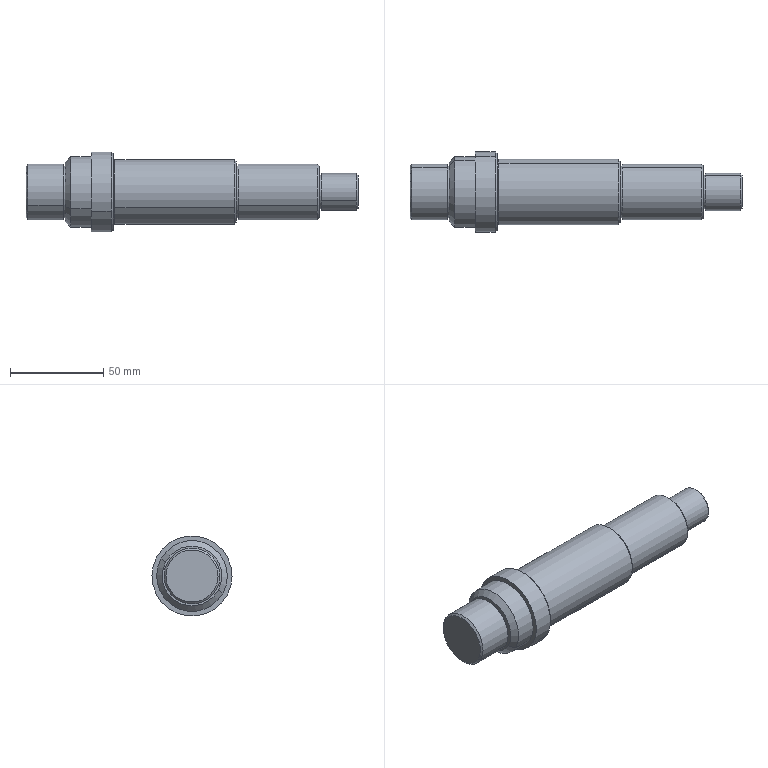Part | STEP file | 20316-1 | 1 solid | 43 faces | box 178 x 43 x 43 mm | volume 148101 mm3 | cylinder 20 | cone 12 | plane 11 | commonest cylinder face diameters 28 x4 30 x4 18 x2 20 x2 33 x2 35 x2
STEP:
#1=CARTESIAN_POINT('',(-19.8,7.898,4.315));
#2=VERTEX_POINT('',#1);
#3=CARTESIAN_POINT('',(-19.8,-7.898,-4.315));
#4=VERTEX_POINT('',#3);
#5=CARTESIAN_POINT('',(-19.8,0.,0.));
#6=DIRECTION('',(1.,0.,0.));
#7=AXIS2_PLACEMENT_3D('',#5,#6,$);
#8=CIRCLE('',#7,9.);
#9=EDGE_CURVE('',#2,#4,#8,.T.);
#10=ORIENTED_EDGE('',*,*,#9,.F.);
#11=CARTESIAN_POINT('',(-20.8,7.898,4.315));
#12=VERTEX_POINT('',#11);
#13=CARTESIAN_POINT('',(-20.3,7.898,4.315));
#14=DIRECTION('',(1.,0.,0.));
#15=VECTOR('',#14,1.);
#16=LINE('',#13,#15);
#17=EDGE_CURVE('',#2,#12,#16,.F.);
#18=ORIENTED_EDGE('',*,*,#17,.T.);
#19=CARTESIAN_POINT('',(-20.8,-7.898,-4.315));
#20=VERTEX_POINT('',#19);
#21=CARTESIAN_POINT('',(-20.8,0.,0.));
#22=DIRECTION('',(1.,0.,0.));
#23=AXIS2_PLACEMENT_3D('',#21,#22,$);
#24=CIRCLE('',#23,9.);
#25=EDGE_CURVE('',#12,#20,#24,.T.);
#26=ORIENTED_EDGE('',*,*,#25,.T.);
#27=CARTESIAN_POINT('',(-20.3,-7.898,-4.315));
#28=DIRECTION('',(1.,0.,0.));
#29=VECTOR('',#28,1.);
#30=LINE('',#27,#29);
#31=EDGE_CURVE('',#4,#20,#30,.F.);
#32=ORIENTED_EDGE('',*,*,#31,.F.);
#33=EDGE_LOOP('',(#10,#18,#26,#32));
#34=FACE_OUTER_BOUND('',#33,.T.);
#35=CARTESIAN_POINT('',(-89.,0.,0.));
#36=DIRECTION('',(1.,0.,0.));
#37=DIRECTION('',(0.,0.8776,0.4794));
#38=AXIS2_PLACEMENT_3D('',#35,#36,#37);
#39=CYLINDRICAL_SURFACE('',#38,9.);
#40=ADVANCED_FACE('',(#34),#39,.T.);
#41=CARTESIAN_POINT('',(-19.8,0.,0.));
#42=DIRECTION('',(1.,0.,0.));
#43=AXIS2_PLACEMENT_3D('',#41,#42,$);
#44=CIRCLE('',#43,9.);
#45=EDGE_CURVE('',#4,#2,#44,.T.);
#46=ORIENTED_EDGE('',*,*,#45,.F.);
#47=ORIENTED_EDGE('',*,*,#31,.T.);
#48=CARTESIAN_POINT('',(-20.8,0.,0.));
#49=DIRECTION('',(1.,0.,0.));
#50=AXIS2_PLACEMENT_3D('',#48,#49,$);
#51=CIRCLE('',#50,9.);
#52=EDGE_CURVE('',#20,#12,#51,.T.);
#53=ORIENTED_EDGE('',*,*,#52,.T.);
#54=ORIENTED_EDGE('',*,*,#17,.F.);
#55=EDGE_LOOP('',(#46,#47,#53,#54));
#56=FACE_OUTER_BOUND('',#55,.T.);
#57=ADVANCED_FACE('',(#56),#39,.T.);
#58=CARTESIAN_POINT('',(-64.3,12.286,6.712));
#59=VERTEX_POINT('',#58);
#60=CARTESIAN_POINT('',(-64.3,-12.286,-6.712));
#61=VERTEX_POINT('',#60);
#62=CARTESIAN_POINT('',(-64.3,0.,0.));
#63=DIRECTION('',(1.,0.,0.));
#64=AXIS2_PLACEMENT_3D('',#62,#63,$);
#65=CIRCLE('',#64,14.);
#66=EDGE_CURVE('',#59,#61,#65,.T.);
#67=ORIENTED_EDGE('',*,*,#66,.F.);
#68=CARTESIAN_POINT('',(-65.3,12.286,6.712));
#69=VERTEX_POINT('',#68);
#70=CARTESIAN_POINT('',(-111.15,12.286,6.712));
#71=DIRECTION('',(1.,0.,0.));
#72=VECTOR('',#71,1.);
#73=LINE('',#70,#72);
#74=EDGE_CURVE('',#59,#69,#73,.F.);
#75=ORIENTED_EDGE('',*,*,#74,.T.);
#76=CARTESIAN_POINT('',(-65.3,-12.286,-6.712));
#77=VERTEX_POINT('',#76);
#78=CARTESIAN_POINT('',(-65.3,0.,0.));
#79=DIRECTION('',(1.,0.,0.));
#80=AXIS2_PLACEMENT_3D('',#78,#79,$);
#81=CIRCLE('',#80,14.);
#82=EDGE_CURVE('',#69,#77,#81,.T.);
#83=ORIENTED_EDGE('',*,*,#82,.T.);
#84=CARTESIAN_POINT('',(-111.15,-12.286,-6.712));
#85=DIRECTION('',(1.,0.,0.));
#86=VECTOR('',#85,1.);
#87=LINE('',#84,#86);
#88=EDGE_CURVE('',#61,#77,#87,.F.);
#89=ORIENTED_EDGE('',*,*,#88,.F.);
#90=EDGE_LOOP('',(#67,#75,#83,#89));
#91=FACE_OUTER_BOUND('',#90,.T.);
#92=CARTESIAN_POINT('',(-89.,0.,0.));
#93=DIRECTION('',(1.,0.,0.));
#94=DIRECTION('',(0.,0.8776,0.4794));
#95=AXIS2_PLACEMENT_3D('',#92,#93,#94);
#96=CYLINDRICAL_SURFACE('',#95,14.);
#97=ADVANCED_FACE('',(#91),#96,.T.);
#98=CARTESIAN_POINT('',(-64.3,0.,0.));
#99=DIRECTION('',(1.,0.,0.));
#100=AXIS2_PLACEMENT_3D('',#98,#99,$);
#101=CIRCLE('',#100,14.);
#102=EDGE_CURVE('',#61,#59,#101,.T.);
#103=ORIENTED_EDGE('',*,*,#102,.F.);
#104=ORIENTED_EDGE('',*,*,#88,.T.);
#105=CARTESIAN_POINT('',(-65.3,0.,0.));
#106=DIRECTION('',(1.,0.,0.));
#107=AXIS2_PLACEMENT_3D('',#105,#106,$);
#108=CIRCLE('',#107,14.);
#109=EDGE_CURVE('',#77,#69,#108,.T.);
#110=ORIENTED_EDGE('',*,*,#109,.T.);
#111=ORIENTED_EDGE('',*,*,#74,.F.);
#112=EDGE_LOOP('',(#103,#104,#110,#111));
#113=FACE_OUTER_BOUND('',#112,.T.);
#114=ADVANCED_FACE('',(#113),#96,.T.);
#115=CARTESIAN_POINT('',(-130.3,14.48,7.911));
#116=VERTEX_POINT('',#115);
#117=CARTESIAN_POINT('',(-130.3,-14.48,-7.911));
#118=VERTEX_POINT('',#117);
#119=CARTESIAN_POINT('',(-130.3,0.,0.));
#120=DIRECTION('',(1.,0.,0.));
#121=AXIS2_PLACEMENT_3D('',#119,#120,$);
#122=CIRCLE('',#121,16.5);
#123=EDGE_CURVE('',#116,#118,#122,.T.);
#124=ORIENTED_EDGE('',*,*,#123,.F.);
#125=CARTESIAN_POINT('',(-131.3,14.48,7.911));
#126=VERTEX_POINT('',#125);
#127=CARTESIAN_POINT('',(-130.8,14.48,7.911));
#128=DIRECTION('',(1.,0.,0.));
#129=VECTOR('',#128,1.);
#130=LINE('',#127,#129);
#131=EDGE_CURVE('',#116,#126,#130,.F.);
#132=ORIENTED_EDGE('',*,*,#131,.T.);
#133=CARTESIAN_POINT('',(-131.3,-14.48,-7.911));
#134=VERTEX_POINT('',#133);
#135=CARTESIAN_POINT('',(-131.3,0.,0.));
#136=DIRECTION('',(1.,0.,0.));
#137=AXIS2_PLACEMENT_3D('',#135,#136,$);
#138=CIRCLE('',#137,16.5);
#139=EDGE_CURVE('',#126,#134,#138,.T.);
#140=ORIENTED_EDGE('',*,*,#139,.T.);
#141=CARTESIAN_POINT('',(-130.8,-14.48,-7.911));
#142=DIRECTION('',(1.,0.,0.));
#143=VECTOR('',#142,1.);
#144=LINE('',#141,#143);
#145=EDGE_CURVE('',#118,#134,#144,.F.);
#146=ORIENTED_EDGE('',*,*,#145,.F.);
#147=EDGE_LOOP('',(#124,#132,#140,#146));
#148=FACE_OUTER_BOUND('',#147,.T.);
#149=CARTESIAN_POINT('',(-89.,0.,0.));
#150=DIRECTION('',(1.,0.,0.));
#151=DIRECTION('',(0.,0.8776,0.4794));
#152=AXIS2_PLACEMENT_3D('',#149,#150,#151);
#153=CYLINDRICAL_SURFACE('',#152,16.5);
#154=ADVANCED_FACE('',(#148),#153,.T.);
#155=CARTESIAN_POINT('',(-130.3,0.,0.));
#156=DIRECTION('',(1.,0.,0.));
#157=AXIS2_PLACEMENT_3D('',#155,#156,$);
#158=CIRCLE('',#157,16.5);
#159=EDGE_CURVE('',#118,#116,#158,.T.);
#160=ORIENTED_EDGE('',*,*,#159,.F.);
#161=ORIENTED_EDGE('',*,*,#145,.T.);
#162=CARTESIAN_POINT('',(-131.3,0.,0.));
#163=DIRECTION('',(1.,0.,0.));
#164=AXIS2_PLACEMENT_3D('',#162,#163,$);
#165=CIRCLE('',#164,16.5);
#166=EDGE_CURVE('',#134,#126,#165,.T.);
#167=ORIENTED_EDGE('',*,*,#166,.T.);
#168=ORIENTED_EDGE('',*,*,#131,.F.);
#169=EDGE_LOOP('',(#160,#161,#167,#168));
#170=FACE_OUTER_BOUND('',#169,.T.);
#171=ADVANCED_FACE('',(#170),#153,.T.);
#172=CARTESIAN_POINT('',(-157.,12.286,6.712));
#173=VERTEX_POINT('',#172);
#174=CARTESIAN_POINT('',(-157.,-12.286,-6.712));
#175=VERTEX_POINT('',#174);
#176=CARTESIAN_POINT('',(-157.,0.,0.));
#177=DIRECTION('',(1.,0.,0.));
#178=AXIS2_PLACEMENT_3D('',#176,#177,$);
#179=CIRCLE('',#178,14.);
#180=EDGE_CURVE('',#173,#175,#179,.T.);
#181=ORIENTED_EDGE('',*,*,#180,.F.);
#182=CARTESIAN_POINT('',(-158.,12.286,6.712));
#183=VERTEX_POINT('',#182);
#184=CARTESIAN_POINT('',(-111.15,12.286,6.712));
#185=DIRECTION('',(1.,0.,0.));
#186=VECTOR('',#185,1.);
#187=LINE('',#184,#186);
#188=EDGE_CURVE('',#173,#183,#187,.F.);
#189=ORIENTED_EDGE('',*,*,#188,.T.);
#190=CARTESIAN_POINT('',(-158.,-12.286,-6.712));
#191=VERTEX_POINT('',#190);
#192=CARTESIAN_POINT('',(-158.,0.,0.));
#193=DIRECTION('',(1.,0.,0.));
#194=AXIS2_PLACEMENT_3D('',#192,#193,$);
#195=CIRCLE('',#194,14.);
#196=EDGE_CURVE('',#183,#191,#195,.T.);
#197=ORIENTED_EDGE('',*,*,#196,.T.);
#198=CARTESIAN_POINT('',(-111.15,-12.286,-6.712));
#199=DIRECTION('',(1.,0.,0.));
#200=VECTOR('',#199,1.);
#201=LINE('',#198,#200);
#202=EDGE_CURVE('',#175,#191,#201,.F.);
#203=ORIENTED_EDGE('',*,*,#202,.F.);
#204=EDGE_LOOP('',(#181,#189,#197,#203));
#205=FACE_OUTER_BOUND('',#204,.T.);
#206=ADVANCED_FACE('',(#205),#96,.T.);
#207=CARTESIAN_POINT('',(-157.,0.,0.));
#208=DIRECTION('',(1.,0.,0.));
#209=AXIS2_PLACEMENT_3D('',#207,#208,$);
#210=CIRCLE('',#209,14.);
#211=EDGE_CURVE('',#175,#173,#210,.T.);
#212=ORIENTED_EDGE('',*,*,#211,.F.);
#213=ORIENTED_EDGE('',*,*,#202,.T.);
#214=CARTESIAN_POINT('',(-158.,0.,0.));
#215=DIRECTION('',(1.,0.,0.));
#216=AXIS2_PLACEMENT_3D('',#214,#215,$);
#217=CIRCLE('',#216,14.);
#218=EDGE_CURVE('',#191,#183,#217,.T.);
#219=ORIENTED_EDGE('',*,*,#218,.T.);
#220=ORIENTED_EDGE('',*,*,#188,.F.);
#221=EDGE_LOOP('',(#212,#213,#219,#220));
#222=FACE_OUTER_BOUND('',#221,.T.);
#223=ADVANCED_FACE('',(#222),#96,.T.);
#224=CARTESIAN_POINT('',(-19.8,8.776,4.794));
#225=VERTEX_POINT('',#224);
#226=CARTESIAN_POINT('',(-19.8,-8.776,-4.794));
#227=VERTEX_POINT('',#226);
#228=CARTESIAN_POINT('',(-19.8,0.,0.));
#229=DIRECTION('',(1.,0.,0.));
#230=AXIS2_PLACEMENT_3D('',#228,#229,$);
#231=CIRCLE('',#230,10.);
#232=EDGE_CURVE('',#225,#227,#231,.T.);
#233=ORIENTED_EDGE('',*,*,#232,.F.);
#234=CARTESIAN_POINT('',(-19.8,0.,0.));
#235=DIRECTION('',(1.,0.,0.));
#236=AXIS2_PLACEMENT_3D('',#234,#235,$);
#237=CIRCLE('',#236,10.);
#238=EDGE_CURVE('',#227,#225,#237,.T.);
#239=ORIENTED_EDGE('',*,*,#238,.F.);
#240=EDGE_LOOP('',(#233,#239));
#241=FACE_OUTER_BOUND('',#240,.T.);
#242=ORIENTED_EDGE('',*,*,#45,.T.);
#243=ORIENTED_EDGE('',*,*,#9,.T.);
#244=EDGE_LOOP('',(#242,#243));
#245=FACE_BOUND('',#244,.T.);
#246=CARTESIAN_POINT('',(-19.8,10.,0.));
#247=DIRECTION('',(1.,0.,0.));
#248=DIRECTION('',(0.,1.,0.));
#249=AXIS2_PLACEMENT_3D('',#246,#247,#248);
#250=PLANE('',#249);
#251=ADVANCED_FACE('',(#241,#245),#250,.F.);
#252=CARTESIAN_POINT('',(-64.3,13.164,7.191));
#253=VERTEX_POINT('',#252);
#254=CARTESIAN_POINT('',(-64.3,-13.164,-7.191));
#255=VERTEX_POINT('',#254);
#256=CARTESIAN_POINT('',(-64.3,0.,0.));
#257=DIRECTION('',(1.,0.,0.));
#258=AXIS2_PLACEMENT_3D('',#256,#257,$);
#259=CIRCLE('',#258,15.);
#260=EDGE_CURVE('',#253,#255,#259,.T.);
#261=ORIENTED_EDGE('',*,*,#260,.F.);
#262=CARTESIAN_POINT('',(-64.3,0.,0.));
#263=DIRECTION('',(1.,0.,0.));
#264=AXIS2_PLACEMENT_3D('',#262,#263,$);
#265=CIRCLE('',#264,15.);
#266=EDGE_CURVE('',#255,#253,#265,.T.);
#267=ORIENTED_EDGE('',*,*,#266,.F.);
#268=EDGE_LOOP('',(#261,#267));
#269=FACE_OUTER_BOUND('',#268,.T.);
#270=ORIENTED_EDGE('',*,*,#102,.T.);
#271=ORIENTED_EDGE('',*,*,#66,.T.);
#272=EDGE_LOOP('',(#270,#271));
#273=FACE_BOUND('',#272,.T.);
#274=CARTESIAN_POINT('',(-64.3,15.,0.));
#275=DIRECTION('',(1.,0.,0.));
#276=DIRECTION('',(0.,1.,0.));
#277=AXIS2_PLACEMENT_3D('',#274,#275,#276);
#278=PLANE('',#277);
#279=ADVANCED_FACE('',(#269,#273),#278,.F.);
#280=CARTESIAN_POINT('',(-130.3,15.358,8.39));
#281=VERTEX_POINT('',#280);
#282=CARTESIAN_POINT('',(-130.3,-15.358,-8.39));
#283=VERTEX_POINT('',#282);
#284=CARTESIAN_POINT('',(-130.3,0.,0.));
#285=DIRECTION('',(1.,0.,0.));
#286=AXIS2_PLACEMENT_3D('',#284,#285,$);
#287=CIRCLE('',#286,17.5);
#288=EDGE_CURVE('',#281,#283,#287,.T.);
#289=ORIENTED_EDGE('',*,*,#288,.F.);
#290=CARTESIAN_POINT('',(-130.3,0.,0.));
#291=DIRECTION('',(1.,0.,0.));
#292=AXIS2_PLACEMENT_3D('',#290,#291,$);
#293=CIRCLE('',#292,17.5);
#294=EDGE_CURVE('',#283,#281,#293,.T.);
#295=ORIENTED_EDGE('',*,*,#294,.F.);
#296=EDGE_LOOP('',(#289,#295));
#297=FACE_OUTER_BOUND('',#296,.T.);
#298=ORIENTED_EDGE('',*,*,#159,.T.);
#299=ORIENTED_EDGE('',*,*,#123,.T.);
#300=EDGE_LOOP('',(#298,#299));
#301=FACE_BOUND('',#300,.T.);
#302=CARTESIAN_POINT('',(-130.3,17.5,0.));
#303=DIRECTION('',(1.,0.,0.));
#304=DIRECTION('',(0.,1.,0.));
#305=AXIS2_PLACEMENT_3D('',#302,#303,#304);
#306=PLANE('',#305);
#307=ADVANCED_FACE('',(#297,#301),#306,.F.);
#308=CARTESIAN_POINT('',(-143.,18.868,10.308));
#309=VERTEX_POINT('',#308);
#310=CARTESIAN_POINT('',(-143.,-18.868,-10.308));
#311=VERTEX_POINT('',#310);
#312=CARTESIAN_POINT('',(-143.,0.,0.));
#313=DIRECTION('',(1.,0.,0.));
#314=AXIS2_PLACEMENT_3D('',#312,#313,$);
#315=CIRCLE('',#314,21.5);
#316=EDGE_CURVE('',#309,#311,#315,.T.);
#317=ORIENTED_EDGE('',*,*,#316,.F.);
#318=CARTESIAN_POINT('',(-143.,0.,0.));
#319=DIRECTION('',(1.,0.,0.));
#320=AXIS2_PLACEMENT_3D('',#318,#319,$);
#321=CIRCLE('',#320,21.5);
#322=EDGE_CURVE('',#311,#309,#321,.T.);
#323=ORIENTED_EDGE('',*,*,#322,.F.);
#324=EDGE_LOOP('',(#317,#323));
#325=FACE_OUTER_BOUND('',#324,.T.);
#326=CARTESIAN_POINT('',(-143.,-16.674,-9.109));
#327=VERTEX_POINT('',#326);
#328=CARTESIAN_POINT('',(-143.,16.674,9.109));
#329=VERTEX_POINT('',#328);
#330=CARTESIAN_POINT('',(-143.,0.,0.));
#331=DIRECTION('',(1.,0.,0.));
#332=AXIS2_PLACEMENT_3D('',#330,#331,$);
#333=CIRCLE('',#332,19.);
#334=EDGE_CURVE('',#327,#329,#333,.T.);
#335=ORIENTED_EDGE('',*,*,#334,.T.);
#336=CARTESIAN_POINT('',(-143.,0.,0.));
#337=DIRECTION('',(1.,0.,0.));
#338=AXIS2_PLACEMENT_3D('',#336,#337,$);
#339=CIRCLE('',#338,19.);
#340=EDGE_CURVE('',#329,#327,#339,.T.);
#341=ORIENTED_EDGE('',*,*,#340,.T.);
#342=EDGE_LOOP('',(#335,#341));
#343=FACE_BOUND('',#342,.T.);
#344=CARTESIAN_POINT('',(-143.,21.5,0.));
#345=DIRECTION('',(1.,0.,0.));
#346=DIRECTION('',(0.,1.,0.));
#347=AXIS2_PLACEMENT_3D('',#344,#345,#346);
#348=PLANE('',#347);
#349=ADVANCED_FACE('',(#325,#343),#348,.F.);
#350=CARTESIAN_POINT('',(-158.,-13.164,-7.191));
#351=VERTEX_POINT('',#350);
#352=CARTESIAN_POINT('',(-158.,13.164,7.191));
#353=VERTEX_POINT('',#352);
#354=CARTESIAN_POINT('',(-158.,0.,0.));
#355=DIRECTION('',(1.,0.,0.));
#356=AXIS2_PLACEMENT_3D('',#354,#355,$);
#357=CIRCLE('',#356,15.);
#358=EDGE_CURVE('',#351,#353,#357,.T.);
#359=ORIENTED_EDGE('',*,*,#358,.T.);
#360=CARTESIAN_POINT('',(-158.,0.,0.));
#361=DIRECTION('',(1.,0.,0.));
#362=AXIS2_PLACEMENT_3D('',#360,#361,$);
#363=CIRCLE('',#362,15.);
#364=EDGE_CURVE('',#353,#351,#363,.T.);
#365=ORIENTED_EDGE('',*,*,#364,.T.);
#366=EDGE_LOOP('',(#359,#365));
#367=FACE_OUTER_BOUND('',#366,.T.);
#368=ORIENTED_EDGE('',*,*,#196,.F.);
#369=ORIENTED_EDGE('',*,*,#218,.F.);
#370=EDGE_LOOP('',(#368,#369));
#371=FACE_BOUND('',#370,.T.);
#372=CARTESIAN_POINT('',(-158.,15.,0.));
#373=DIRECTION('',(1.,0.,0.));
#374=DIRECTION('',(0.,1.,0.));
#375=AXIS2_PLACEMENT_3D('',#372,#373,#374);
#376=PLANE('',#375);
#377=ADVANCED_FACE('',(#367,#371),#376,.T.);
#378=CARTESIAN_POINT('',(-177.,-13.164,-7.191));
#379=VERTEX_POINT('',#378);
#380=CARTESIAN_POINT('',(-99.4,-13.164,-7.191));
#381=DIRECTION('',(1.,0.,0.));
#382=VECTOR('',#381,1.);
#383=LINE('',#380,#382);
#384=EDGE_CURVE('',#351,#379,#383,.F.);
#385=ORIENTED_EDGE('',*,*,#384,.F.);
#386=ORIENTED_EDGE('',*,*,#364,.F.);
#387=CARTESIAN_POINT('',(-177.,13.164,7.191));
#388=VERTEX_POINT('',#387);
#389=CARTESIAN_POINT('',(-99.4,13.164,7.191));
#390=DIRECTION('',(1.,0.,0.));
#391=VECTOR('',#390,1.);
#392=LINE('',#389,#391);
#393=EDGE_CURVE('',#353,#388,#392,.F.);
#394=ORIENTED_EDGE('',*,*,#393,.T.);
#395=CARTESIAN_POINT('',(-177.,0.,0.));
#396=DIRECTION('',(1.,0.,0.));
#397=AXIS2_PLACEMENT_3D('',#395,#396,$);
#398=CIRCLE('',#397,15.);
#399=EDGE_CURVE('',#388,#379,#398,.T.);
#400=ORIENTED_EDGE('',*,*,#399,.T.);
#401=EDGE_LOOP('',(#385,#386,#394,#400));
#402=FACE_OUTER_BOUND('',#401,.T.);
#403=CARTESIAN_POINT('',(-89.,0.,0.));
#404=DIRECTION('',(1.,0.,0.));
#405=DIRECTION('',(0.,0.8776,0.4794));
#406=AXIS2_PLACEMENT_3D('',#403,#404,#405);
#407=CYLINDRICAL_SURFACE('',#406,15.);
#408=ADVANCED_FACE('',(#402),#407,.T.);
#409=ORIENTED_EDGE('',*,*,#393,.F.);
#410=ORIENTED_EDGE('',*,*,#358,.F.);
#411=ORIENTED_EDGE('',*,*,#384,.T.);
#412=CARTESIAN_POINT('',(-177.,0.,0.));
#413=DIRECTION('',(1.,0.,0.));
#414=AXIS2_PLACEMENT_3D('',#412,#413,$);
#415=CIRCLE('',#414,15.);
#416=EDGE_CURVE('',#379,#388,#415,.T.);
#417=ORIENTED_EDGE('',*,*,#416,.T.);
#418=EDGE_LOOP('',(#409,#410,#411,#417));
#419=FACE_OUTER_BOUND('',#418,.T.);
#420=ADVANCED_FACE('',(#419),#407,.T.);
#421=CARTESIAN_POINT('',(-178.,12.286,6.712));
#422=VERTEX_POINT('',#421);
#423=CARTESIAN_POINT('',(-178.,-12.286,-6.712));
#424=VERTEX_POINT('',#423);
#425=CARTESIAN_POINT('',(-178.,0.,0.));
#426=DIRECTION('',(1.,0.,0.));
#427=AXIS2_PLACEMENT_3D('',#425,#426,$);
#428=CIRCLE('',#427,14.);
#429=EDGE_CURVE('',#422,#424,#428,.T.);
#430=ORIENTED_EDGE('',*,*,#429,.F.);
#431=CARTESIAN_POINT('',(-178.,0.,0.));
#432=DIRECTION('',(1.,0.,0.));
#433=AXIS2_PLACEMENT_3D('',#431,#432,$);
#434=CIRCLE('',#433,14.);
#435=EDGE_CURVE('',#424,#422,#434,.T.);
#436=ORIENTED_EDGE('',*,*,#435,.F.);
#437=EDGE_LOOP('',(#430,#436));
#438=FACE_OUTER_BOUND('',#437,.T.);
#439=CARTESIAN_POINT('',(-178.,15.,0.));
#440=DIRECTION('',(1.,0.,0.));
#441=DIRECTION('',(0.,1.,0.));
#442=AXIS2_PLACEMENT_3D('',#439,#440,#441);
#443=PLANE('',#442);
#444=ADVANCED_FACE('',(#438),#443,.F.);
#445=CARTESIAN_POINT('',(-177.5,-12.725,-6.952));
#446=DIRECTION('',(0.7071,-0.6205,-0.339));
#447=VECTOR('',#446,1.);
#448=LINE('',#445,#447);
#449=EDGE_CURVE('',#379,#424,#448,.F.);
#450=ORIENTED_EDGE('',*,*,#449,.T.);
#451=ORIENTED_EDGE('',*,*,#435,.T.);
#452=CARTESIAN_POINT('',(-177.5,12.725,6.952));
#453=DIRECTION('',(0.7071,0.6205,0.339));
#454=VECTOR('',#453,1.);
#455=LINE('',#452,#454);
#456=EDGE_CURVE('',#388,#422,#455,.F.);
#457=ORIENTED_EDGE('',*,*,#456,.F.);
#458=ORIENTED_EDGE('',*,*,#416,.F.);
#459=EDGE_LOOP('',(#450,#451,#457,#458));
#460=FACE_OUTER_BOUND('',#459,.T.);
#461=CARTESIAN_POINT('',(-192.,0.,0.));
#462=DIRECTION('',(1.,0.,0.));
#463=DIRECTION('',(0.,-0.8958,-0.4444));
#464=AXIS2_PLACEMENT_3D('',#461,#462,#463);
#465=CONICAL_SURFACE('',#464,0.,0.7854);
#466=ADVANCED_FACE('',(#460),#465,.T.);
#467=ORIENTED_EDGE('',*,*,#456,.T.);
#468=ORIENTED_EDGE('',*,*,#429,.T.);
#469=ORIENTED_EDGE('',*,*,#449,.F.);
#470=ORIENTED_EDGE('',*,*,#399,.F.);
#471=EDGE_LOOP('',(#467,#468,#469,#470));
#472=FACE_OUTER_BOUND('',#471,.T.);
#473=CARTESIAN_POINT('',(-192.,0.,0.));
#474=DIRECTION('',(1.,0.,0.));
#475=DIRECTION('',(0.,0.8776,0.4794));
#476=AXIS2_PLACEMENT_3D('',#473,#474,#475);
#477=CONICAL_SURFACE('',#476,0.,0.7854);
#478=ADVANCED_FACE('',(#472),#477,.T.);
#479=CARTESIAN_POINT('',(-132.3,18.868,10.308));
#480=VERTEX_POINT('',#479);
#481=CARTESIAN_POINT('',(-137.15,18.868,10.308));
#482=DIRECTION('',(1.,0.,0.));
#483=VECTOR('',#482,1.);
#484=LINE('',#481,#483);
#485=EDGE_CURVE('',#480,#309,#484,.F.);
#486=ORIENTED_EDGE('',*,*,#485,.T.);
#487=ORIENTED_EDGE('',*,*,#316,.T.);
#488=CARTESIAN_POINT('',(-132.3,-18.868,-10.308));
#489=VERTEX_POINT('',#488);
#490=CARTESIAN_POINT('',(-137.15,-18.868,-10.308));
#491=DIRECTION('',(1.,0.,0.));
#492=VECTOR('',#491,1.);
#493=LINE('',#490,#492);
#494=EDGE_CURVE('',#489,#311,#493,.F.);
#495=ORIENTED_EDGE('',*,*,#494,.F.);
#496=CARTESIAN_POINT('',(-132.3,0.,0.));
#497=DIRECTION('',(1.,0.,0.));
#498=AXIS2_PLACEMENT_3D('',#496,#497,$);
#499=CIRCLE('',#498,21.5);
#500=EDGE_CURVE('',#480,#489,#499,.T.);
#501=ORIENTED_EDGE('',*,*,#500,.F.);
#502=EDGE_LOOP('',(#486,#487,#495,#501));
#503=FACE_OUTER_BOUND('',#502,.T.);
#504=CARTESIAN_POINT('',(-89.,0.,0.));
#505=DIRECTION('',(1.,0.,0.));
#506=DIRECTION('',(0.,0.8776,0.4794));
#507=AXIS2_PLACEMENT_3D('',#504,#505,#506);
#508=CYLINDRICAL_SURFACE('',#507,21.5);
#509=ADVANCED_FACE('',(#503),#508,.T.);
#510=ORIENTED_EDGE('',*,*,#494,.T.);
#511=ORIENTED_EDGE('',*,*,#322,.T.);
#512=ORIENTED_EDGE('',*,*,#485,.F.);
#513=CARTESIAN_POINT('',(-132.3,0.,0.));
#514=DIRECTION('',(1.,0.,0.));
#515=AXIS2_PLACEMENT_3D('',#513,#514,$);
#516=CIRCLE('',#515,21.5);
#517=EDGE_CURVE('',#489,#480,#516,.T.);
#518=ORIENTED_EDGE('',*,*,#517,.F.);
#519=EDGE_LOOP('',(#510,#511,#512,#518));
#520=FACE_OUTER_BOUND('',#519,.T.);
#521=ADVANCED_FACE('',(#520),#508,.T.);
#522=CARTESIAN_POINT('',(-131.3,-17.99,-9.828));
#523=VERTEX_POINT('',#522);
#524=CARTESIAN_POINT('',(-131.3,17.99,9.828));
#525=VERTEX_POINT('',#524);
#526=CARTESIAN_POINT('',(-131.3,0.,0.));
#527=DIRECTION('',(1.,0.,0.));
#528=AXIS2_PLACEMENT_3D('',#526,#527,$);
#529=CIRCLE('',#528,20.5);
#530=EDGE_CURVE('',#523,#525,#529,.T.);
#531=ORIENTED_EDGE('',*,*,#530,.T.);
#532=CARTESIAN_POINT('',(-131.3,0.,0.));
#533=DIRECTION('',(1.,0.,0.));
#534=AXIS2_PLACEMENT_3D('',#532,#533,$);
#535=CIRCLE('',#534,20.5);
#536=EDGE_CURVE('',#525,#523,#535,.T.);
#537=ORIENTED_EDGE('',*,*,#536,.T.);
#538=EDGE_LOOP('',(#531,#537));
#539=FACE_OUTER_BOUND('',#538,.T.);
#540=ORIENTED_EDGE('',*,*,#139,.F.);
#541=ORIENTED_EDGE('',*,*,#166,.F.);
#542=EDGE_LOOP('',(#540,#541));
#543=FACE_BOUND('',#542,.T.);
#544=CARTESIAN_POINT('',(-131.3,16.5,0.));
#545=DIRECTION('',(1.,0.,0.));
#546=DIRECTION('',(0.,1.,0.));
#547=AXIS2_PLACEMENT_3D('',#544,#545,#546);
#548=PLANE('',#547);
#549=ADVANCED_FACE('',(#539,#543),#548,.T.);
#550=CARTESIAN_POINT('',(-131.8,-18.429,-10.068));
#551=DIRECTION('',(-0.7071,-0.6205,-0.339));
#552=VECTOR('',#551,1.);
#553=LINE('',#550,#552);
#554=EDGE_CURVE('',#523,#489,#553,.T.);
#555=ORIENTED_EDGE('',*,*,#554,.T.);
#556=ORIENTED_EDGE('',*,*,#517,.T.);
#557=CARTESIAN_POINT('',(-131.8,18.429,10.068));
#558=DIRECTION('',(-0.7071,0.6205,0.339));
#559=VECTOR('',#558,1.);
#560=LINE('',#557,#559);
#561=EDGE_CURVE('',#525,#480,#560,.T.);
#562=ORIENTED_EDGE('',*,*,#561,.F.);
#563=ORIENTED_EDGE('',*,*,#530,.F.);
#564=EDGE_LOOP('',(#555,#556,#562,#563));
#565=FACE_OUTER_BOUND('',#564,.T.);
#566=CARTESIAN_POINT('',(-110.8,0.,0.));
#567=DIRECTION('',(-1.,0.,0.));
#568=DIRECTION('',(0.,-0.9997,-0.0256));
#569=AXIS2_PLACEMENT_3D('',#566,#567,#568);
#570=CONICAL_SURFACE('',#569,0.,0.7854);
#571=ADVANCED_FACE('',(#565),#570,.T.);
#572=ORIENTED_EDGE('',*,*,#561,.T.);
#573=ORIENTED_EDGE('',*,*,#500,.T.);
#574=ORIENTED_EDGE('',*,*,#554,.F.);
#575=ORIENTED_EDGE('',*,*,#536,.F.);
#576=EDGE_LOOP('',(#572,#573,#574,#575));
#577=FACE_OUTER_BOUND('',#576,.T.);
#578=CARTESIAN_POINT('',(-110.8,0.,0.));
#579=DIRECTION('',(-1.,0.,0.));
#580=DIRECTION('',(0.,0.8776,0.4794));
#581=AXIS2_PLACEMENT_3D('',#578,#579,#580);
#582=CONICAL_SURFACE('',#581,0.,0.7854);
#583=ADVANCED_FACE('',(#577),#582,.T.);
#584=CARTESIAN_POINT('',(-66.3,15.358,8.39));
#585=VERTEX_POINT('',#584);
#586=CARTESIAN_POINT('',(-97.8,15.358,8.39));
#587=DIRECTION('',(1.,0.,0.));
#588=VECTOR('',#587,1.);
#589=LINE('',#586,#588);
#590=EDGE_CURVE('',#585,#281,#589,.F.);
#591=ORIENTED_EDGE('',*,*,#590,.T.);
#592=ORIENTED_EDGE('',*,*,#288,.T.);
#593=CARTESIAN_POINT('',(-66.3,-15.358,-8.39));
#594=VERTEX_POINT('',#593);
#595=CARTESIAN_POINT('',(-97.8,-15.358,-8.39));
#596=DIRECTION('',(1.,0.,0.));
#597=VECTOR('',#596,1.);
#598=LINE('',#595,#597);
#599=EDGE_CURVE('',#594,#283,#598,.F.);
#600=ORIENTED_EDGE('',*,*,#599,.F.);
#601=CARTESIAN_POINT('',(-66.3,0.,0.));
#602=DIRECTION('',(1.,0.,0.));
#603=AXIS2_PLACEMENT_3D('',#601,#602,$);
#604=CIRCLE('',#603,17.5);
#605=EDGE_CURVE('',#585,#594,#604,.T.);
#606=ORIENTED_EDGE('',*,*,#605,.F.);
#607=EDGE_LOOP('',(#591,#592,#600,#606));
#608=FACE_OUTER_BOUND('',#607,.T.);
#609=CARTESIAN_POINT('',(-89.,0.,0.));
#610=DIRECTION('',(1.,0.,0.));
#611=DIRECTION('',(0.,0.8776,0.4794));
#612=AXIS2_PLACEMENT_3D('',#609,#610,#611);
#613=CYLINDRICAL_SURFACE('',#612,17.5);
#614=ADVANCED_FACE('',(#608),#613,.T.);
#615=ORIENTED_EDGE('',*,*,#599,.T.);
#616=ORIENTED_EDGE('',*,*,#294,.T.);
#617=ORIENTED_EDGE('',*,*,#590,.F.);
#618=CARTESIAN_POINT('',(-66.3,0.,0.));
#619=DIRECTION('',(1.,0.,0.));
#620=AXIS2_PLACEMENT_3D('',#618,#619,$);
#621=CIRCLE('',#620,17.5);
#622=EDGE_CURVE('',#594,#585,#621,.T.);
#623=ORIENTED_EDGE('',*,*,#622,.F.);
#624=EDGE_LOOP('',(#615,#616,#617,#623));
#625=FACE_OUTER_BOUND('',#624,.T.);
#626=ADVANCED_FACE('',(#625),#613,.T.);
#627=CARTESIAN_POINT('',(-65.3,-14.48,-7.911));
#628=VERTEX_POINT('',#627);
#629=CARTESIAN_POINT('',(-65.3,14.48,7.911));
#630=VERTEX_POINT('',#629);
#631=CARTESIAN_POINT('',(-65.3,0.,0.));
#632=DIRECTION('',(1.,0.,0.));
#633=AXIS2_PLACEMENT_3D('',#631,#632,$);
#634=CIRCLE('',#633,16.5);
#635=EDGE_CURVE('',#628,#630,#634,.T.);
#636=ORIENTED_EDGE('',*,*,#635,.T.);
#637=CARTESIAN_POINT('',(-65.3,0.,0.));
#638=DIRECTION('',(1.,0.,0.));
#639=AXIS2_PLACEMENT_3D('',#637,#638,$);
#640=CIRCLE('',#639,16.5);
#641=EDGE_CURVE('',#630,#628,#640,.T.);
#642=ORIENTED_EDGE('',*,*,#641,.T.);
#643=EDGE_LOOP('',(#636,#642));
#644=FACE_OUTER_BOUND('',#643,.T.);
#645=ORIENTED_EDGE('',*,*,#82,.F.);
#646=ORIENTED_EDGE('',*,*,#109,.F.);
#647=EDGE_LOOP('',(#645,#646));
#648=FACE_BOUND('',#647,.T.);
#649=CARTESIAN_POINT('',(-65.3,14.,0.));
#650=DIRECTION('',(1.,0.,0.));
#651=DIRECTION('',(0.,1.,0.));
#652=AXIS2_PLACEMENT_3D('',#649,#650,#651);
#653=PLANE('',#652);
#654=ADVANCED_FACE('',(#644,#648),#653,.T.);
#655=CARTESIAN_POINT('',(-65.8,-14.919,-8.15));
#656=DIRECTION('',(-0.7071,-0.6205,-0.339));
#657=VECTOR('',#656,1.);
#658=LINE('',#655,#657);
#659=EDGE_CURVE('',#628,#594,#658,.T.);
#660=ORIENTED_EDGE('',*,*,#659,.T.);
#661=ORIENTED_EDGE('',*,*,#622,.T.);
#662=CARTESIAN_POINT('',(-65.8,14.919,8.15));
#663=DIRECTION('',(-0.7071,0.6205,0.339));
#664=VECTOR('',#663,1.);
#665=LINE('',#662,#664);
#666=EDGE_CURVE('',#630,#585,#665,.T.);
#667=ORIENTED_EDGE('',*,*,#666,.F.);
#668=ORIENTED_EDGE('',*,*,#635,.F.);
#669=EDGE_LOOP('',(#660,#661,#667,#668));
#670=FACE_OUTER_BOUND('',#669,.T.);
#671=CARTESIAN_POINT('',(-48.8,0.,0.));
#672=DIRECTION('',(-1.,0.,0.));
#673=DIRECTION('',(0.,-0.8897,-0.4566));
#674=AXIS2_PLACEMENT_3D('',#671,#672,#673);
#675=CONICAL_SURFACE('',#674,0.,0.7854);
#676=ADVANCED_FACE('',(#670),#675,.T.);
#677=ORIENTED_EDGE('',*,*,#666,.T.);
#678=ORIENTED_EDGE('',*,*,#605,.T.);
#679=ORIENTED_EDGE('',*,*,#659,.F.);
#680=ORIENTED_EDGE('',*,*,#641,.F.);
#681=EDGE_LOOP('',(#677,#678,#679,#680));
#682=FACE_OUTER_BOUND('',#681,.T.);
#683=CARTESIAN_POINT('',(-48.8,0.,0.));
#684=DIRECTION('',(-1.,0.,0.));
#685=DIRECTION('',(0.,0.8776,0.4794));
#686=AXIS2_PLACEMENT_3D('',#683,#684,#685);
#687=CONICAL_SURFACE('',#686,0.,0.7854);
#688=ADVANCED_FACE('',(#682),#687,.T.);
#689=CARTESIAN_POINT('',(-21.8,13.164,7.191));
#690=VERTEX_POINT('',#689);
#691=CARTESIAN_POINT('',(-99.4,13.164,7.191));
#692=DIRECTION('',(1.,0.,0.));
#693=VECTOR('',#692,1.);
#694=LINE('',#691,#693);
#695=EDGE_CURVE('',#690,#253,#694,.F.);
#696=ORIENTED_EDGE('',*,*,#695,.T.);
#697=ORIENTED_EDGE('',*,*,#260,.T.);
#698=CARTESIAN_POINT('',(-21.8,-13.164,-7.191));
#699=VERTEX_POINT('',#698);
#700=CARTESIAN_POINT('',(-99.4,-13.164,-7.191));
#701=DIRECTION('',(1.,0.,0.));
#702=VECTOR('',#701,1.);
#703=LINE('',#700,#702);
#704=EDGE_CURVE('',#699,#255,#703,.F.);
#705=ORIENTED_EDGE('',*,*,#704,.F.);
#706=CARTESIAN_POINT('',(-21.8,0.,0.));
#707=DIRECTION('',(1.,0.,0.));
#708=AXIS2_PLACEMENT_3D('',#706,#707,$);
#709=CIRCLE('',#708,15.);
#710=EDGE_CURVE('',#690,#699,#709,.T.);
#711=ORIENTED_EDGE('',*,*,#710,.F.);
#712=EDGE_LOOP('',(#696,#697,#705,#711));
#713=FACE_OUTER_BOUND('',#712,.T.);
#714=ADVANCED_FACE('',(#713),#407,.T.);
#715=ORIENTED_EDGE('',*,*,#704,.T.);
#716=ORIENTED_EDGE('',*,*,#266,.T.);
#717=ORIENTED_EDGE('',*,*,#695,.F.);
#718=CARTESIAN_POINT('',(-21.8,0.,0.));
#719=DIRECTION('',(1.,0.,0.));
#720=AXIS2_PLACEMENT_3D('',#718,#719,$);
#721=CIRCLE('',#720,15.);
#722=EDGE_CURVE('',#699,#690,#721,.T.);
#723=ORIENTED_EDGE('',*,*,#722,.F.);
#724=EDGE_LOOP('',(#715,#716,#717,#723));
#725=FACE_OUTER_BOUND('',#724,.T.);
#726=ADVANCED_FACE('',(#725),#407,.T.);
#727=CARTESIAN_POINT('',(-20.8,-12.286,-6.712));
#728=VERTEX_POINT('',#727);
#729=CARTESIAN_POINT('',(-20.8,12.286,6.712));
#730=VERTEX_POINT('',#729);
#731=CARTESIAN_POINT('',(-20.8,0.,0.));
#732=DIRECTION('',(1.,0.,0.));
#733=AXIS2_PLACEMENT_3D('',#731,#732,$);
#734=CIRCLE('',#733,14.);
#735=EDGE_CURVE('',#728,#730,#734,.T.);
#736=ORIENTED_EDGE('',*,*,#735,.T.);
#737=CARTESIAN_POINT('',(-20.8,0.,0.));
#738=DIRECTION('',(1.,0.,0.));
#739=AXIS2_PLACEMENT_3D('',#737,#738,$);
#740=CIRCLE('',#739,14.);
#741=EDGE_CURVE('',#730,#728,#740,.T.);
#742=ORIENTED_EDGE('',*,*,#741,.T.);
#743=EDGE_LOOP('',(#736,#742));
#744=FACE_OUTER_BOUND('',#743,.T.);
#745=ORIENTED_EDGE('',*,*,#25,.F.);
#746=ORIENTED_EDGE('',*,*,#52,.F.);
#747=EDGE_LOOP('',(#745,#746));
#748=FACE_BOUND('',#747,.T.);
#749=CARTESIAN_POINT('',(-20.8,9.,0.));
#750=DIRECTION('',(1.,0.,0.));
#751=DIRECTION('',(0.,1.,0.));
#752=AXIS2_PLACEMENT_3D('',#749,#750,#751);
#753=PLANE('',#752);
#754=ADVANCED_FACE('',(#744,#748),#753,.T.);
#755=CARTESIAN_POINT('',(-21.3,-12.725,-6.952));
#756=DIRECTION('',(-0.7071,-0.6205,-0.339));
#757=VECTOR('',#756,1.);
#758=LINE('',#755,#757);
#759=EDGE_CURVE('',#728,#699,#758,.T.);
#760=ORIENTED_EDGE('',*,*,#759,.T.);
#761=ORIENTED_EDGE('',*,*,#722,.T.);
#762=CARTESIAN_POINT('',(-21.3,12.725,6.952));
#763=DIRECTION('',(-0.7071,0.6205,0.339));
#764=VECTOR('',#763,1.);
#765=LINE('',#762,#764);
#766=EDGE_CURVE('',#730,#690,#765,.T.);
#767=ORIENTED_EDGE('',*,*,#766,.F.);
#768=ORIENTED_EDGE('',*,*,#735,.F.);
#769=EDGE_LOOP('',(#760,#761,#767,#768));
#770=FACE_OUTER_BOUND('',#769,.T.);
#771=CARTESIAN_POINT('',(-6.8,0.,0.));
#772=DIRECTION('',(-1.,0.,0.));
#773=DIRECTION('',(0.,-0.9961,-0.08875));
#774=AXIS2_PLACEMENT_3D('',#771,#772,#773);
#775=CONICAL_SURFACE('',#774,0.,0.7854);
#776=ADVANCED_FACE('',(#770),#775,.T.);
#777=ORIENTED_EDGE('',*,*,#766,.T.);
#778=ORIENTED_EDGE('',*,*,#710,.T.);
#779=ORIENTED_EDGE('',*,*,#759,.F.);
#780=ORIENTED_EDGE('',*,*,#741,.F.);
#781=EDGE_LOOP('',(#777,#778,#779,#780));
#782=FACE_OUTER_BOUND('',#781,.T.);
#783=CARTESIAN_POINT('',(-6.8,0.,0.));
#784=DIRECTION('',(-1.,0.,0.));
#785=DIRECTION('',(0.,0.8776,0.4794));
#786=AXIS2_PLACEMENT_3D('',#783,#784,#785);
#787=CONICAL_SURFACE('',#786,0.,0.7854);
#788=ADVANCED_FACE('',(#782),#787,.T.);
#789=CARTESIAN_POINT('',(-1.,8.776,4.794));
#790=VERTEX_POINT('',#789);
#791=CARTESIAN_POINT('',(-9.9,8.776,4.794));
#792=DIRECTION('',(1.,0.,0.));
#793=VECTOR('',#792,1.);
#794=LINE('',#791,#793);
#795=EDGE_CURVE('',#790,#225,#794,.F.);
#796=ORIENTED_EDGE('',*,*,#795,.T.);
#797=ORIENTED_EDGE('',*,*,#232,.T.);
#798=CARTESIAN_POINT('',(-1.,-8.776,-4.794));
#799=VERTEX_POINT('',#798);
#800=CARTESIAN_POINT('',(-9.9,-8.776,-4.794));
#801=DIRECTION('',(1.,0.,0.));
#802=VECTOR('',#801,1.);
#803=LINE('',#800,#802);
#804=EDGE_CURVE('',#799,#227,#803,.F.);
#805=ORIENTED_EDGE('',*,*,#804,.F.);
#806=CARTESIAN_POINT('',(-1.,0.,0.));
#807=DIRECTION('',(1.,0.,0.));
#808=AXIS2_PLACEMENT_3D('',#806,#807,$);
#809=CIRCLE('',#808,10.);
#810=EDGE_CURVE('',#790,#799,#809,.T.);
#811=ORIENTED_EDGE('',*,*,#810,.F.);
#812=EDGE_LOOP('',(#796,#797,#805,#811));
#813=FACE_OUTER_BOUND('',#812,.T.);
#814=CARTESIAN_POINT('',(-89.,0.,0.));
#815=DIRECTION('',(1.,0.,0.));
#816=DIRECTION('',(0.,0.8776,0.4794));
#817=AXIS2_PLACEMENT_3D('',#814,#815,#816);
#818=CYLINDRICAL_SURFACE('',#817,10.);
#819=ADVANCED_FACE('',(#813),#818,.T.);
#820=ORIENTED_EDGE('',*,*,#804,.T.);
#821=ORIENTED_EDGE('',*,*,#238,.T.);
#822=ORIENTED_EDGE('',*,*,#795,.F.);
#823=CARTESIAN_POINT('',(-1.,0.,0.));
#824=DIRECTION('',(1.,0.,0.));
#825=AXIS2_PLACEMENT_3D('',#823,#824,$);
#826=CIRCLE('',#825,10.);
#827=EDGE_CURVE('',#799,#790,#826,.T.);
#828=ORIENTED_EDGE('',*,*,#827,.F.);
#829=EDGE_LOOP('',(#820,#821,#822,#828));
#830=FACE_OUTER_BOUND('',#829,.T.);
#831=ADVANCED_FACE('',(#830),#818,.T.);
#832=CARTESIAN_POINT('',(0.,7.898,4.315));
#833=VERTEX_POINT('',#832);
#834=CARTESIAN_POINT('',(0.,-7.898,-4.315));
#835=VERTEX_POINT('',#834);
#836=CARTESIAN_POINT('',(0.,0.,0.));
#837=DIRECTION('',(1.,0.,0.));
#838=AXIS2_PLACEMENT_3D('',#836,#837,$);
#839=CIRCLE('',#838,9.);
#840=EDGE_CURVE('',#833,#835,#839,.T.);
#841=ORIENTED_EDGE('',*,*,#840,.T.);
#842=CARTESIAN_POINT('',(0.,0.,0.));
#843=DIRECTION('',(1.,0.,0.));
#844=AXIS2_PLACEMENT_3D('',#842,#843,$);
#845=CIRCLE('',#844,9.);
#846=EDGE_CURVE('',#835,#833,#845,.T.);
#847=ORIENTED_EDGE('',*,*,#846,.T.);
#848=EDGE_LOOP('',(#841,#847));
#849=FACE_OUTER_BOUND('',#848,.T.);
#850=CARTESIAN_POINT('',(0.,0.,0.));
#851=DIRECTION('',(1.,0.,0.));
#852=DIRECTION('',(0.,1.,0.));
#853=AXIS2_PLACEMENT_3D('',#850,#851,#852);
#854=PLANE('',#853);
#855=ADVANCED_FACE('',(#849),#854,.T.);
#856=CARTESIAN_POINT('',(-0.5,8.337,4.555));
#857=DIRECTION('',(-0.7071,0.6205,0.339));
#858=VECTOR('',#857,1.);
#859=LINE('',#856,#858);
#860=EDGE_CURVE('',#833,#790,#859,.T.);
#861=ORIENTED_EDGE('',*,*,#860,.T.);
#862=ORIENTED_EDGE('',*,*,#810,.T.);
#863=CARTESIAN_POINT('',(-0.5,-8.337,-4.555));
#864=DIRECTION('',(-0.7071,-0.6205,-0.339));
#865=VECTOR('',#864,1.);
#866=LINE('',#863,#865);
#867=EDGE_CURVE('',#835,#799,#866,.T.);
#868=ORIENTED_EDGE('',*,*,#867,.F.);
#869=ORIENTED_EDGE('',*,*,#840,.F.);
#870=EDGE_LOOP('',(#861,#862,#868,#869));
#871=FACE_OUTER_BOUND('',#870,.T.);
#872=CARTESIAN_POINT('',(9.,0.,0.));
#873=DIRECTION('',(-1.,0.,0.));
#874=DIRECTION('',(0.,0.8776,0.4794));
#875=AXIS2_PLACEMENT_3D('',#872,#873,#874);
#876=CONICAL_SURFACE('',#875,0.,0.7854);
#877=ADVANCED_FACE('',(#871),#876,.T.);
#878=ORIENTED_EDGE('',*,*,#867,.T.);
#879=ORIENTED_EDGE('',*,*,#827,.T.);
#880=ORIENTED_EDGE('',*,*,#860,.F.);
#881=ORIENTED_EDGE('',*,*,#846,.F.);
#882=EDGE_LOOP('',(#878,#879,#880,#881));
#883=FACE_OUTER_BOUND('',#882,.T.);
#884=CARTESIAN_POINT('',(9.,0.,0.));
#885=DIRECTION('',(-1.,0.,0.));
#886=DIRECTION('',(0.,-0.9409,-0.3387));
#887=AXIS2_PLACEMENT_3D('',#884,#885,#886);
#888=CONICAL_SURFACE('',#887,0.,0.7854);
#889=ADVANCED_FACE('',(#883),#888,.T.);
#890=CARTESIAN_POINT('',(-154.,-16.674,-9.109));
#891=VERTEX_POINT('',#890);
#892=CARTESIAN_POINT('',(-150.,-16.674,-9.109));
#893=DIRECTION('',(1.,0.,0.));
#894=VECTOR('',#893,1.);
#895=LINE('',#892,#894);
#896=EDGE_CURVE('',#327,#891,#895,.F.);
#897=ORIENTED_EDGE('',*,*,#896,.F.);
#898=ORIENTED_EDGE('',*,*,#340,.F.);
#899=CARTESIAN_POINT('',(-154.,16.674,9.109));
#900=VERTEX_POINT('',#899);
#901=CARTESIAN_POINT('',(-150.,16.674,9.109));
#902=DIRECTION('',(1.,0.,0.));
#903=VECTOR('',#902,1.);
#904=LINE('',#901,#903);
#905=EDGE_CURVE('',#329,#900,#904,.F.);
#906=ORIENTED_EDGE('',*,*,#905,.T.);
#907=CARTESIAN_POINT('',(-154.,0.,0.));
#908=DIRECTION('',(1.,0.,0.));
#909=AXIS2_PLACEMENT_3D('',#907,#908,$);
#910=CIRCLE('',#909,19.);
#911=EDGE_CURVE('',#900,#891,#910,.T.);
#912=ORIENTED_EDGE('',*,*,#911,.T.);
#913=EDGE_LOOP('',(#897,#898,#906,#912));
#914=FACE_OUTER_BOUND('',#913,.T.);
#915=CARTESIAN_POINT('',(-89.,0.,0.));
#916=DIRECTION('',(1.,0.,0.));
#917=DIRECTION('',(0.,0.8776,0.4794));
#918=AXIS2_PLACEMENT_3D('',#915,#916,#917);
#919=CYLINDRICAL_SURFACE('',#918,19.);
#920=ADVANCED_FACE('',(#914),#919,.T.);
#921=ORIENTED_EDGE('',*,*,#905,.F.);
#922=ORIENTED_EDGE('',*,*,#334,.F.);
#923=ORIENTED_EDGE('',*,*,#896,.T.);
#924=CARTESIAN_POINT('',(-154.,0.,0.));
#925=DIRECTION('',(1.,0.,0.));
#926=AXIS2_PLACEMENT_3D('',#924,#925,$);
#927=CIRCLE('',#926,19.);
#928=EDGE_CURVE('',#891,#900,#927,.T.);
#929=ORIENTED_EDGE('',*,*,#928,.T.);
#930=EDGE_LOOP('',(#921,#922,#923,#929));
#931=FACE_OUTER_BOUND('',#930,.T.);
#932=ADVANCED_FACE('',(#931),#919,.T.);
#933=CARTESIAN_POINT('',(-157.,14.041,7.671));
#934=VERTEX_POINT('',#933);
#935=CARTESIAN_POINT('',(-157.,-14.041,-7.671));
#936=VERTEX_POINT('',#935);
#937=CARTESIAN_POINT('',(-157.,0.,0.));
#938=DIRECTION('',(1.,0.,0.));
#939=AXIS2_PLACEMENT_3D('',#937,#938,$);
#940=CIRCLE('',#939,16.);
#941=EDGE_CURVE('',#934,#936,#940,.T.);
#942=ORIENTED_EDGE('',*,*,#941,.F.);
#943=CARTESIAN_POINT('',(-157.,0.,0.));
#944=DIRECTION('',(1.,0.,0.));
#945=AXIS2_PLACEMENT_3D('',#943,#944,$);
#946=CIRCLE('',#945,16.);
#947=EDGE_CURVE('',#936,#934,#946,.T.);
#948=ORIENTED_EDGE('',*,*,#947,.F.);
#949=EDGE_LOOP('',(#942,#948));
#950=FACE_OUTER_BOUND('',#949,.T.);
#951=ORIENTED_EDGE('',*,*,#211,.T.);
#952=ORIENTED_EDGE('',*,*,#180,.T.);
#953=EDGE_LOOP('',(#951,#952));
#954=FACE_BOUND('',#953,.T.);
#955=CARTESIAN_POINT('',(-157.,19.,0.));
#956=DIRECTION('',(1.,0.,0.));
#957=DIRECTION('',(0.,1.,0.));
#958=AXIS2_PLACEMENT_3D('',#955,#956,#957);
#959=PLANE('',#958);
#960=ADVANCED_FACE('',(#950,#954),#959,.F.);
#961=CARTESIAN_POINT('',(-155.5,-15.358,-8.39));
#962=DIRECTION('',(0.7071,-0.6205,-0.339));
#963=VECTOR('',#962,1.);
#964=LINE('',#961,#963);
#965=EDGE_CURVE('',#891,#936,#964,.F.);
#966=ORIENTED_EDGE('',*,*,#965,.T.);
#967=ORIENTED_EDGE('',*,*,#947,.T.);
#968=CARTESIAN_POINT('',(-155.5,15.358,8.39));
#969=DIRECTION('',(0.7071,0.6205,0.339));
#970=VECTOR('',#969,1.);
#971=LINE('',#968,#970);
#972=EDGE_CURVE('',#900,#934,#971,.F.);
#973=ORIENTED_EDGE('',*,*,#972,.F.);
#974=ORIENTED_EDGE('',*,*,#928,.F.);
#975=EDGE_LOOP('',(#966,#967,#973,#974));
#976=FACE_OUTER_BOUND('',#975,.T.);
#977=CARTESIAN_POINT('',(-173.,0.,0.));
#978=DIRECTION('',(1.,0.,0.));
#979=DIRECTION('',(0.,-0.9763,-0.2165));
#980=AXIS2_PLACEMENT_3D('',#977,#978,#979);
#981=CONICAL_SURFACE('',#980,0.,0.7854);
#982=ADVANCED_FACE('',(#976),#981,.T.);
#983=ORIENTED_EDGE('',*,*,#972,.T.);
#984=ORIENTED_EDGE('',*,*,#941,.T.);
#985=ORIENTED_EDGE('',*,*,#965,.F.);
#986=ORIENTED_EDGE('',*,*,#911,.F.);
#987=EDGE_LOOP('',(#983,#984,#985,#986));
#988=FACE_OUTER_BOUND('',#987,.T.);
#989=CARTESIAN_POINT('',(-173.,0.,0.));
#990=DIRECTION('',(1.,0.,0.));
#991=DIRECTION('',(0.,0.8776,0.4794));
#992=AXIS2_PLACEMENT_3D('',#989,#990,#991);
#993=CONICAL_SURFACE('',#992,0.,0.7854);
#994=ADVANCED_FACE('',(#988),#993,.T.);
#995=CLOSED_SHELL('',(#40,#57,#97,#114,#154,#171,#206,#223,#251,#279,#307,#349,#377,#408,#420,#444,#466,#478,#509,#521,#549,#571,#583,#614,#626,#654,#676,#688,#714,#726,#754,#776,#788,#819,#831,#855,#877,#889,#920,#932,#960,#982,#994));
#996=MANIFOLD_SOLID_BREP('',#995);
#997=(LENGTH_UNIT()NAMED_UNIT(*)SI_UNIT(.MILLI.,.METRE.));
#998=UNCERTAINTY_MEASURE_WITH_UNIT(LENGTH_MEASURE(0.005),#997,'','');
#999=(NAMED_UNIT(*)PLANE_ANGLE_UNIT()SI_UNIT($,.RADIAN.));
#1000=(NAMED_UNIT(*)SI_UNIT($,.STERADIAN.)SOLID_ANGLE_UNIT());
#1001=(GEOMETRIC_REPRESENTATION_CONTEXT(3)GLOBAL_UNCERTAINTY_ASSIGNED_CONTEXT((#998))GLOBAL_UNIT_ASSIGNED_CONTEXT((#997,#999,#1000))REPRESENTATION_CONTEXT('',''));
#1002=ADVANCED_BREP_SHAPE_REPRESENTATION('',(#996),#1001);